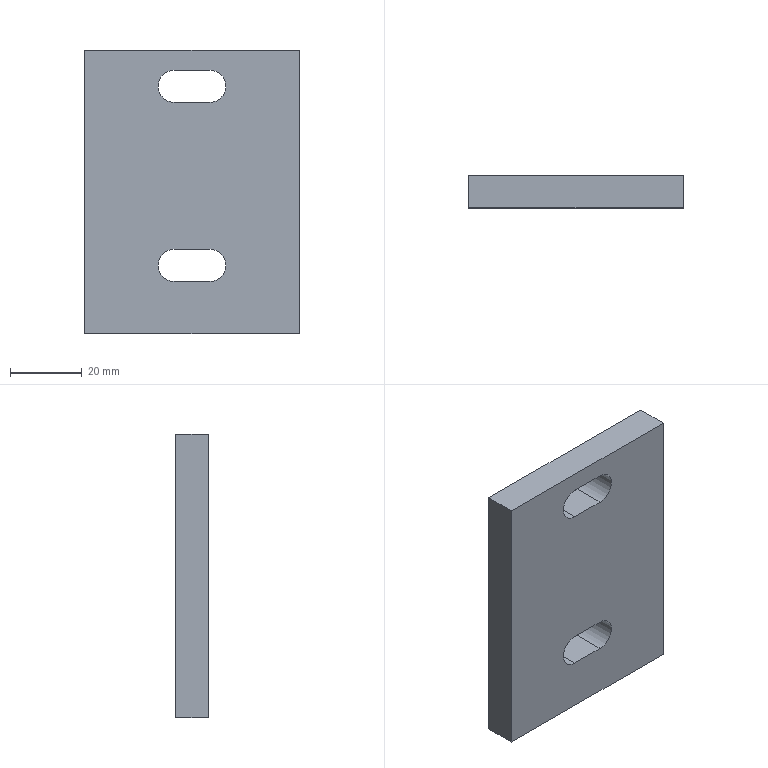Part | STEP file | X77-03212 | 1 solid | 14 faces | box 60 x 9 x 79 mm | volume 39895 mm3 | plane 10 | cylinder 4 | commonest cylinder face diameters 9 x4
STEP:
#1=CARTESIAN_POINT('',(-189.937,-72.716,80.));
#2=VERTEX_POINT('',#1);
#3=CARTESIAN_POINT('',(-189.937,-72.716,1.));
#4=VERTEX_POINT('',#3);
#5=CARTESIAN_POINT('',(-189.937,-72.716,80.));
#6=DIRECTION('',(0.,0.,-1.));
#7=VECTOR('',#6,1000.);
#8=LINE('',#5,#7);
#9=EDGE_CURVE('',#2,#4,#8,.T.);
#10=ORIENTED_EDGE('',*,*,#9,.T.);
#11=CARTESIAN_POINT('',(-189.937,-81.716,1.));
#12=VERTEX_POINT('',#11);
#13=CARTESIAN_POINT('',(-189.937,-72.716,1.));
#14=DIRECTION('',(0.,-1.,0.));
#15=VECTOR('',#14,1000.);
#16=LINE('',#13,#15);
#17=EDGE_CURVE('',#4,#12,#16,.T.);
#18=ORIENTED_EDGE('',*,*,#17,.T.);
#19=CARTESIAN_POINT('',(-189.937,-81.716,80.));
#20=VERTEX_POINT('',#19);
#21=CARTESIAN_POINT('',(-189.937,-81.716,80.));
#22=DIRECTION('',(0.,0.,1.));
#23=VECTOR('',#22,1000.);
#24=LINE('',#21,#23);
#25=EDGE_CURVE('',#12,#20,#24,.T.);
#26=ORIENTED_EDGE('',*,*,#25,.T.);
#27=CARTESIAN_POINT('',(-189.937,-72.716,80.));
#28=DIRECTION('',(0.,-1.,0.));
#29=VECTOR('',#28,1000.);
#30=LINE('',#27,#29);
#31=EDGE_CURVE('',#2,#20,#30,.T.);
#32=ORIENTED_EDGE('',*,*,#31,.F.);
#33=EDGE_LOOP('',(#10,#18,#26,#32));
#34=FACE_OUTER_BOUND('',#33,.T.);
#35=CARTESIAN_POINT('',(-189.937,-72.716,80.));
#36=DIRECTION('',(1.,0.,0.));
#37=DIRECTION('',(0.,0.,-1.));
#38=AXIS2_PLACEMENT_3D('',#35,#36,#37);
#39=PLANE('',#38);
#40=ADVANCED_FACE('',(#34),#39,.F.);
#41=CARTESIAN_POINT('',(-129.937,-81.716,80.));
#42=VERTEX_POINT('',#41);
#43=CARTESIAN_POINT('',(-129.937,-81.716,1.));
#44=VERTEX_POINT('',#43);
#45=CARTESIAN_POINT('',(-129.937,-81.716,80.));
#46=DIRECTION('',(0.,0.,-1.));
#47=VECTOR('',#46,1000.);
#48=LINE('',#45,#47);
#49=EDGE_CURVE('',#42,#44,#48,.T.);
#50=ORIENTED_EDGE('',*,*,#49,.T.);
#51=CARTESIAN_POINT('',(-129.937,-72.716,1.));
#52=VERTEX_POINT('',#51);
#53=CARTESIAN_POINT('',(-129.937,-72.716,1.));
#54=DIRECTION('',(0.,1.,0.));
#55=VECTOR('',#54,1000.);
#56=LINE('',#53,#55);
#57=EDGE_CURVE('',#44,#52,#56,.T.);
#58=ORIENTED_EDGE('',*,*,#57,.T.);
#59=CARTESIAN_POINT('',(-129.937,-72.716,80.));
#60=VERTEX_POINT('',#59);
#61=CARTESIAN_POINT('',(-129.937,-72.716,80.));
#62=DIRECTION('',(0.,0.,-1.));
#63=VECTOR('',#62,1000.);
#64=LINE('',#61,#63);
#65=EDGE_CURVE('',#60,#52,#64,.T.);
#66=ORIENTED_EDGE('',*,*,#65,.F.);
#67=CARTESIAN_POINT('',(-129.937,-72.716,80.));
#68=DIRECTION('',(0.,1.,0.));
#69=VECTOR('',#68,1000.);
#70=LINE('',#67,#69);
#71=EDGE_CURVE('',#42,#60,#70,.T.);
#72=ORIENTED_EDGE('',*,*,#71,.F.);
#73=EDGE_LOOP('',(#50,#58,#66,#72));
#74=FACE_OUTER_BOUND('',#73,.T.);
#75=CARTESIAN_POINT('',(-129.937,-72.716,80.));
#76=DIRECTION('',(-1.,0.,0.));
#77=DIRECTION('',(0.,0.,1.));
#78=AXIS2_PLACEMENT_3D('',#75,#76,#77);
#79=PLANE('',#78);
#80=ADVANCED_FACE('',(#74),#79,.F.);
#81=CARTESIAN_POINT('',(-164.937,-72.716,24.5));
#82=VERTEX_POINT('',#81);
#83=CARTESIAN_POINT('',(-154.937,-72.716,24.5));
#84=VERTEX_POINT('',#83);
#85=CARTESIAN_POINT('',(-164.937,-72.716,24.5));
#86=DIRECTION('',(1.,0.,0.));
#87=VECTOR('',#86,1000.);
#88=LINE('',#85,#87);
#89=EDGE_CURVE('',#82,#84,#88,.T.);
#90=ORIENTED_EDGE('',*,*,#89,.F.);
#91=CARTESIAN_POINT('',(-164.937,-72.716,15.5));
#92=VERTEX_POINT('',#91);
#93=CARTESIAN_POINT('',(-164.937,-72.716,20.));
#94=DIRECTION('',(0.,1.,0.));
#95=DIRECTION('',(0.,0.,1.));
#96=AXIS2_PLACEMENT_3D('',#93,#94,#95);
#97=CIRCLE('',#96,4.5);
#98=EDGE_CURVE('',#92,#82,#97,.T.);
#99=ORIENTED_EDGE('',*,*,#98,.F.);
#100=CARTESIAN_POINT('',(-154.937,-72.716,15.5));
#101=VERTEX_POINT('',#100);
#102=CARTESIAN_POINT('',(-164.937,-72.716,15.5));
#103=DIRECTION('',(-1.,0.,0.));
#104=VECTOR('',#103,1000.);
#105=LINE('',#102,#104);
#106=EDGE_CURVE('',#101,#92,#105,.T.);
#107=ORIENTED_EDGE('',*,*,#106,.F.);
#108=CARTESIAN_POINT('',(-154.937,-72.716,20.));
#109=DIRECTION('',(0.,1.,0.));
#110=DIRECTION('',(0.,0.,1.));
#111=AXIS2_PLACEMENT_3D('',#108,#109,#110);
#112=CIRCLE('',#111,4.5);
#113=EDGE_CURVE('',#84,#101,#112,.T.);
#114=ORIENTED_EDGE('',*,*,#113,.F.);
#115=EDGE_LOOP('',(#90,#99,#107,#114));
#116=FACE_BOUND('',#115,.T.);
#117=CARTESIAN_POINT('',(-164.937,-72.716,74.5));
#118=VERTEX_POINT('',#117);
#119=CARTESIAN_POINT('',(-154.937,-72.716,74.5));
#120=VERTEX_POINT('',#119);
#121=CARTESIAN_POINT('',(-164.937,-72.716,74.5));
#122=DIRECTION('',(1.,0.,0.));
#123=VECTOR('',#122,1000.);
#124=LINE('',#121,#123);
#125=EDGE_CURVE('',#118,#120,#124,.T.);
#126=ORIENTED_EDGE('',*,*,#125,.F.);
#127=CARTESIAN_POINT('',(-164.937,-72.716,65.5));
#128=VERTEX_POINT('',#127);
#129=CARTESIAN_POINT('',(-164.937,-72.716,70.));
#130=DIRECTION('',(0.,1.,0.));
#131=DIRECTION('',(0.,0.,1.));
#132=AXIS2_PLACEMENT_3D('',#129,#130,#131);
#133=CIRCLE('',#132,4.5);
#134=EDGE_CURVE('',#128,#118,#133,.T.);
#135=ORIENTED_EDGE('',*,*,#134,.F.);
#136=CARTESIAN_POINT('',(-154.937,-72.716,65.5));
#137=VERTEX_POINT('',#136);
#138=CARTESIAN_POINT('',(-164.937,-72.716,65.5));
#139=DIRECTION('',(-1.,0.,0.));
#140=VECTOR('',#139,1000.);
#141=LINE('',#138,#140);
#142=EDGE_CURVE('',#137,#128,#141,.T.);
#143=ORIENTED_EDGE('',*,*,#142,.F.);
#144=CARTESIAN_POINT('',(-154.937,-72.716,70.));
#145=DIRECTION('',(0.,1.,0.));
#146=DIRECTION('',(0.,0.,1.));
#147=AXIS2_PLACEMENT_3D('',#144,#145,#146);
#148=CIRCLE('',#147,4.5);
#149=EDGE_CURVE('',#120,#137,#148,.T.);
#150=ORIENTED_EDGE('',*,*,#149,.F.);
#151=EDGE_LOOP('',(#126,#135,#143,#150));
#152=FACE_BOUND('',#151,.T.);
#153=ORIENTED_EDGE('',*,*,#65,.T.);
#154=CARTESIAN_POINT('',(-189.937,-72.716,1.));
#155=DIRECTION('',(-1.,0.,0.));
#156=VECTOR('',#155,1000.);
#157=LINE('',#154,#156);
#158=EDGE_CURVE('',#52,#4,#157,.T.);
#159=ORIENTED_EDGE('',*,*,#158,.T.);
#160=ORIENTED_EDGE('',*,*,#9,.F.);
#161=CARTESIAN_POINT('',(-189.937,-72.716,80.));
#162=DIRECTION('',(-1.,0.,0.));
#163=VECTOR('',#162,1000.);
#164=LINE('',#161,#163);
#165=EDGE_CURVE('',#60,#2,#164,.T.);
#166=ORIENTED_EDGE('',*,*,#165,.F.);
#167=EDGE_LOOP('',(#153,#159,#160,#166));
#168=FACE_OUTER_BOUND('',#167,.T.);
#169=CARTESIAN_POINT('',(-189.937,-72.716,80.));
#170=DIRECTION('',(0.,-1.,0.));
#171=DIRECTION('',(0.,0.,-1.));
#172=AXIS2_PLACEMENT_3D('',#169,#170,#171);
#173=PLANE('',#172);
#174=ADVANCED_FACE('',(#116,#152,#168),#173,.F.);
#175=CARTESIAN_POINT('',(-109.937,-81.716,80.));
#176=DIRECTION('',(-1.,0.,0.));
#177=VECTOR('',#176,1000.);
#178=LINE('',#175,#177);
#179=EDGE_CURVE('',#42,#20,#178,.T.);
#180=ORIENTED_EDGE('',*,*,#179,.F.);
#181=ORIENTED_EDGE('',*,*,#71,.T.);
#182=ORIENTED_EDGE('',*,*,#165,.T.);
#183=ORIENTED_EDGE('',*,*,#31,.T.);
#184=EDGE_LOOP('',(#180,#181,#182,#183));
#185=FACE_OUTER_BOUND('',#184,.T.);
#186=CARTESIAN_POINT('',(-189.937,-82.716,80.));
#187=DIRECTION('',(0.,0.,1.));
#188=DIRECTION('',(1.,0.,0.));
#189=AXIS2_PLACEMENT_3D('',#186,#187,#188);
#190=PLANE('',#189);
#191=ADVANCED_FACE('',(#185),#190,.T.);
#192=CARTESIAN_POINT('',(-164.937,-81.716,74.5));
#193=VERTEX_POINT('',#192);
#194=CARTESIAN_POINT('',(-164.937,-82.716,74.5));
#195=DIRECTION('',(0.,1.,0.));
#196=VECTOR('',#195,1000.);
#197=LINE('',#194,#196);
#198=EDGE_CURVE('',#193,#118,#197,.T.);
#199=ORIENTED_EDGE('',*,*,#198,.F.);
#200=CARTESIAN_POINT('',(-164.937,-81.716,65.5));
#201=VERTEX_POINT('',#200);
#202=CARTESIAN_POINT('',(-164.937,-81.716,70.));
#203=DIRECTION('',(0.,-1.,0.));
#204=DIRECTION('',(0.,0.,1.));
#205=AXIS2_PLACEMENT_3D('',#202,#203,#204);
#206=CIRCLE('',#205,4.5);
#207=EDGE_CURVE('',#193,#201,#206,.T.);
#208=ORIENTED_EDGE('',*,*,#207,.T.);
#209=CARTESIAN_POINT('',(-164.937,-82.716,65.5));
#210=DIRECTION('',(0.,1.,0.));
#211=VECTOR('',#210,1000.);
#212=LINE('',#209,#211);
#213=EDGE_CURVE('',#201,#128,#212,.T.);
#214=ORIENTED_EDGE('',*,*,#213,.T.);
#215=ORIENTED_EDGE('',*,*,#134,.T.);
#216=EDGE_LOOP('',(#199,#208,#214,#215));
#217=FACE_OUTER_BOUND('',#216,.T.);
#218=CARTESIAN_POINT('',(-164.937,-82.716,70.));
#219=DIRECTION('',(0.,1.,0.));
#220=DIRECTION('',(0.,0.,1.));
#221=AXIS2_PLACEMENT_3D('',#218,#219,#220);
#222=CYLINDRICAL_SURFACE('',#221,4.5);
#223=ADVANCED_FACE('',(#217),#222,.F.);
#224=ORIENTED_EDGE('',*,*,#213,.F.);
#225=CARTESIAN_POINT('',(-154.937,-81.716,65.5));
#226=VERTEX_POINT('',#225);
#227=CARTESIAN_POINT('',(-164.937,-81.716,65.5));
#228=DIRECTION('',(1.,0.,0.));
#229=VECTOR('',#228,1000.);
#230=LINE('',#227,#229);
#231=EDGE_CURVE('',#201,#226,#230,.T.);
#232=ORIENTED_EDGE('',*,*,#231,.T.);
#233=CARTESIAN_POINT('',(-154.937,-82.716,65.5));
#234=DIRECTION('',(0.,1.,0.));
#235=VECTOR('',#234,1000.);
#236=LINE('',#233,#235);
#237=EDGE_CURVE('',#226,#137,#236,.T.);
#238=ORIENTED_EDGE('',*,*,#237,.T.);
#239=ORIENTED_EDGE('',*,*,#142,.T.);
#240=EDGE_LOOP('',(#224,#232,#238,#239));
#241=FACE_OUTER_BOUND('',#240,.T.);
#242=CARTESIAN_POINT('',(-164.937,-82.716,65.5));
#243=DIRECTION('',(0.,0.,-1.));
#244=DIRECTION('',(-1.,0.,0.));
#245=AXIS2_PLACEMENT_3D('',#242,#243,#244);
#246=PLANE('',#245);
#247=ADVANCED_FACE('',(#241),#246,.F.);
#248=ORIENTED_EDGE('',*,*,#237,.F.);
#249=CARTESIAN_POINT('',(-154.937,-81.716,74.5));
#250=VERTEX_POINT('',#249);
#251=CARTESIAN_POINT('',(-154.937,-81.716,70.));
#252=DIRECTION('',(0.,-1.,0.));
#253=DIRECTION('',(0.,0.,1.));
#254=AXIS2_PLACEMENT_3D('',#251,#252,#253);
#255=CIRCLE('',#254,4.5);
#256=EDGE_CURVE('',#226,#250,#255,.T.);
#257=ORIENTED_EDGE('',*,*,#256,.T.);
#258=CARTESIAN_POINT('',(-154.937,-82.716,74.5));
#259=DIRECTION('',(0.,1.,0.));
#260=VECTOR('',#259,1000.);
#261=LINE('',#258,#260);
#262=EDGE_CURVE('',#250,#120,#261,.T.);
#263=ORIENTED_EDGE('',*,*,#262,.T.);
#264=ORIENTED_EDGE('',*,*,#149,.T.);
#265=EDGE_LOOP('',(#248,#257,#263,#264));
#266=FACE_OUTER_BOUND('',#265,.T.);
#267=CARTESIAN_POINT('',(-154.937,-82.716,70.));
#268=DIRECTION('',(0.,1.,0.));
#269=DIRECTION('',(0.,0.,1.));
#270=AXIS2_PLACEMENT_3D('',#267,#268,#269);
#271=CYLINDRICAL_SURFACE('',#270,4.5);
#272=ADVANCED_FACE('',(#266),#271,.F.);
#273=ORIENTED_EDGE('',*,*,#262,.F.);
#274=CARTESIAN_POINT('',(-164.937,-81.716,74.5));
#275=DIRECTION('',(-1.,0.,0.));
#276=VECTOR('',#275,1000.);
#277=LINE('',#274,#276);
#278=EDGE_CURVE('',#250,#193,#277,.T.);
#279=ORIENTED_EDGE('',*,*,#278,.T.);
#280=ORIENTED_EDGE('',*,*,#198,.T.);
#281=ORIENTED_EDGE('',*,*,#125,.T.);
#282=EDGE_LOOP('',(#273,#279,#280,#281));
#283=FACE_OUTER_BOUND('',#282,.T.);
#284=CARTESIAN_POINT('',(-164.937,-82.716,74.5));
#285=DIRECTION('',(0.,0.,1.));
#286=DIRECTION('',(1.,0.,0.));
#287=AXIS2_PLACEMENT_3D('',#284,#285,#286);
#288=PLANE('',#287);
#289=ADVANCED_FACE('',(#283),#288,.F.);
#290=CARTESIAN_POINT('',(-164.937,-81.716,24.5));
#291=VERTEX_POINT('',#290);
#292=CARTESIAN_POINT('',(-164.937,-82.716,24.5));
#293=DIRECTION('',(0.,1.,0.));
#294=VECTOR('',#293,1000.);
#295=LINE('',#292,#294);
#296=EDGE_CURVE('',#291,#82,#295,.T.);
#297=ORIENTED_EDGE('',*,*,#296,.F.);
#298=CARTESIAN_POINT('',(-164.937,-81.716,15.5));
#299=VERTEX_POINT('',#298);
#300=CARTESIAN_POINT('',(-164.937,-81.716,20.));
#301=DIRECTION('',(0.,-1.,0.));
#302=DIRECTION('',(0.,0.,1.));
#303=AXIS2_PLACEMENT_3D('',#300,#301,#302);
#304=CIRCLE('',#303,4.5);
#305=EDGE_CURVE('',#291,#299,#304,.T.);
#306=ORIENTED_EDGE('',*,*,#305,.T.);
#307=CARTESIAN_POINT('',(-164.937,-82.716,15.5));
#308=DIRECTION('',(0.,1.,0.));
#309=VECTOR('',#308,1000.);
#310=LINE('',#307,#309);
#311=EDGE_CURVE('',#299,#92,#310,.T.);
#312=ORIENTED_EDGE('',*,*,#311,.T.);
#313=ORIENTED_EDGE('',*,*,#98,.T.);
#314=EDGE_LOOP('',(#297,#306,#312,#313));
#315=FACE_OUTER_BOUND('',#314,.T.);
#316=CARTESIAN_POINT('',(-164.937,-82.716,20.));
#317=DIRECTION('',(0.,1.,0.));
#318=DIRECTION('',(0.,0.,1.));
#319=AXIS2_PLACEMENT_3D('',#316,#317,#318);
#320=CYLINDRICAL_SURFACE('',#319,4.5);
#321=ADVANCED_FACE('',(#315),#320,.F.);
#322=ORIENTED_EDGE('',*,*,#311,.F.);
#323=CARTESIAN_POINT('',(-154.937,-81.716,15.5));
#324=VERTEX_POINT('',#323);
#325=CARTESIAN_POINT('',(-164.937,-81.716,15.5));
#326=DIRECTION('',(1.,0.,0.));
#327=VECTOR('',#326,1000.);
#328=LINE('',#325,#327);
#329=EDGE_CURVE('',#299,#324,#328,.T.);
#330=ORIENTED_EDGE('',*,*,#329,.T.);
#331=CARTESIAN_POINT('',(-154.937,-82.716,15.5));
#332=DIRECTION('',(0.,1.,0.));
#333=VECTOR('',#332,1000.);
#334=LINE('',#331,#333);
#335=EDGE_CURVE('',#324,#101,#334,.T.);
#336=ORIENTED_EDGE('',*,*,#335,.T.);
#337=ORIENTED_EDGE('',*,*,#106,.T.);
#338=EDGE_LOOP('',(#322,#330,#336,#337));
#339=FACE_OUTER_BOUND('',#338,.T.);
#340=CARTESIAN_POINT('',(-164.937,-82.716,15.5));
#341=DIRECTION('',(0.,0.,-1.));
#342=DIRECTION('',(-1.,0.,0.));
#343=AXIS2_PLACEMENT_3D('',#340,#341,#342);
#344=PLANE('',#343);
#345=ADVANCED_FACE('',(#339),#344,.F.);
#346=ORIENTED_EDGE('',*,*,#335,.F.);
#347=CARTESIAN_POINT('',(-154.937,-81.716,24.5));
#348=VERTEX_POINT('',#347);
#349=CARTESIAN_POINT('',(-154.937,-81.716,20.));
#350=DIRECTION('',(0.,-1.,0.));
#351=DIRECTION('',(0.,0.,1.));
#352=AXIS2_PLACEMENT_3D('',#349,#350,#351);
#353=CIRCLE('',#352,4.5);
#354=EDGE_CURVE('',#324,#348,#353,.T.);
#355=ORIENTED_EDGE('',*,*,#354,.T.);
#356=CARTESIAN_POINT('',(-154.937,-82.716,24.5));
#357=DIRECTION('',(0.,1.,0.));
#358=VECTOR('',#357,1000.);
#359=LINE('',#356,#358);
#360=EDGE_CURVE('',#348,#84,#359,.T.);
#361=ORIENTED_EDGE('',*,*,#360,.T.);
#362=ORIENTED_EDGE('',*,*,#113,.T.);
#363=EDGE_LOOP('',(#346,#355,#361,#362));
#364=FACE_OUTER_BOUND('',#363,.T.);
#365=CARTESIAN_POINT('',(-154.937,-82.716,20.));
#366=DIRECTION('',(0.,1.,0.));
#367=DIRECTION('',(0.,0.,1.));
#368=AXIS2_PLACEMENT_3D('',#365,#366,#367);
#369=CYLINDRICAL_SURFACE('',#368,4.5);
#370=ADVANCED_FACE('',(#364),#369,.F.);
#371=ORIENTED_EDGE('',*,*,#360,.F.);
#372=CARTESIAN_POINT('',(-164.937,-81.716,24.5));
#373=DIRECTION('',(-1.,0.,0.));
#374=VECTOR('',#373,1000.);
#375=LINE('',#372,#374);
#376=EDGE_CURVE('',#348,#291,#375,.T.);
#377=ORIENTED_EDGE('',*,*,#376,.T.);
#378=ORIENTED_EDGE('',*,*,#296,.T.);
#379=ORIENTED_EDGE('',*,*,#89,.T.);
#380=EDGE_LOOP('',(#371,#377,#378,#379));
#381=FACE_OUTER_BOUND('',#380,.T.);
#382=CARTESIAN_POINT('',(-164.937,-82.716,24.5));
#383=DIRECTION('',(0.,0.,1.));
#384=DIRECTION('',(1.,0.,0.));
#385=AXIS2_PLACEMENT_3D('',#382,#383,#384);
#386=PLANE('',#385);
#387=ADVANCED_FACE('',(#381),#386,.F.);
#388=ORIENTED_EDGE('',*,*,#158,.F.);
#389=ORIENTED_EDGE('',*,*,#57,.F.);
#390=CARTESIAN_POINT('',(-109.937,-81.716,1.));
#391=DIRECTION('',(-1.,0.,0.));
#392=VECTOR('',#391,1000.);
#393=LINE('',#390,#392);
#394=EDGE_CURVE('',#44,#12,#393,.T.);
#395=ORIENTED_EDGE('',*,*,#394,.T.);
#396=ORIENTED_EDGE('',*,*,#17,.F.);
#397=EDGE_LOOP('',(#388,#389,#395,#396));
#398=FACE_OUTER_BOUND('',#397,.T.);
#399=CARTESIAN_POINT('',(-109.937,47.284,1.));
#400=DIRECTION('',(0.,0.,1.));
#401=DIRECTION('',(0.,-1.,0.));
#402=AXIS2_PLACEMENT_3D('',#399,#400,#401);
#403=PLANE('',#402);
#404=ADVANCED_FACE('',(#398),#403,.F.);
#405=ORIENTED_EDGE('',*,*,#376,.F.);
#406=ORIENTED_EDGE('',*,*,#354,.F.);
#407=ORIENTED_EDGE('',*,*,#329,.F.);
#408=ORIENTED_EDGE('',*,*,#305,.F.);
#409=EDGE_LOOP('',(#405,#406,#407,#408));
#410=FACE_BOUND('',#409,.T.);
#411=ORIENTED_EDGE('',*,*,#278,.F.);
#412=ORIENTED_EDGE('',*,*,#256,.F.);
#413=ORIENTED_EDGE('',*,*,#231,.F.);
#414=ORIENTED_EDGE('',*,*,#207,.F.);
#415=EDGE_LOOP('',(#411,#412,#413,#414));
#416=FACE_BOUND('',#415,.T.);
#417=ORIENTED_EDGE('',*,*,#394,.F.);
#418=ORIENTED_EDGE('',*,*,#49,.F.);
#419=ORIENTED_EDGE('',*,*,#179,.T.);
#420=ORIENTED_EDGE('',*,*,#25,.F.);
#421=EDGE_LOOP('',(#417,#418,#419,#420));
#422=FACE_OUTER_BOUND('',#421,.T.);
#423=CARTESIAN_POINT('',(-109.937,-81.716,1.));
#424=DIRECTION('',(0.,1.,0.));
#425=DIRECTION('',(0.,0.,1.));
#426=AXIS2_PLACEMENT_3D('',#423,#424,#425);
#427=PLANE('',#426);
#428=ADVANCED_FACE('',(#410,#416,#422),#427,.F.);
#429=CLOSED_SHELL('',(#40,#80,#174,#191,#223,#247,#272,#289,#321,#345,#370,#387,#404,#428));
#430=MANIFOLD_SOLID_BREP('',#429);
#431=CARTESIAN_POINT('',(0.,0.,0.));
#432=DIRECTION('',(0.,0.,1.));
#433=DIRECTION('',(1.,0.,0.));
#434=AXIS2_PLACEMENT_3D('',#431,#432,#433);
#435=(LENGTH_UNIT()NAMED_UNIT(*)SI_UNIT(.MILLI.,.METRE.));
#436=UNCERTAINTY_MEASURE_WITH_UNIT(LENGTH_MEASURE(0.00001),#435,'','');
#437=(NAMED_UNIT(*)PLANE_ANGLE_UNIT()SI_UNIT($,.RADIAN.));
#438=(NAMED_UNIT(*)SI_UNIT($,.STERADIAN.)SOLID_ANGLE_UNIT());
#439=(GEOMETRIC_REPRESENTATION_CONTEXT(3)GLOBAL_UNCERTAINTY_ASSIGNED_CONTEXT((#436))GLOBAL_UNIT_ASSIGNED_CONTEXT((#435,#437,#438))REPRESENTATION_CONTEXT('',''));
#440=ADVANCED_BREP_SHAPE_REPRESENTATION('',(#430,#434),#439);